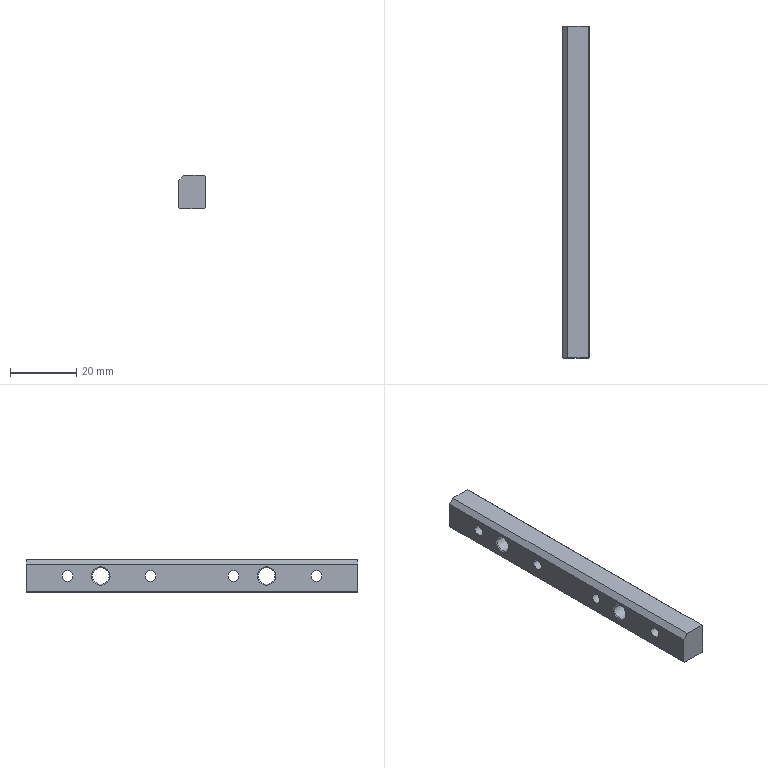Part | NX | 1 solid | 38 faces | box 8 x 100 x 10 mm | volume 7277 mm3 | cone 16 | cylinder 12 | plane 10 | commonest cylinder face diameters 3.3 x8 5 x4
STEP:
#1=CARTESIAN_POINT('',(7.7,0.,0.));
#2=VERTEX_POINT('',#1);
#3=CARTESIAN_POINT('',(1.5,0.,0.));
#4=VERTEX_POINT('',#3);
#5=CARTESIAN_POINT('',(8.,0.,0.));
#6=DIRECTION('',(-1.,0.,0.));
#7=VECTOR('',#6,1000.);
#8=LINE('',#5,#7);
#9=EDGE_CURVE('',#2,#4,#8,.T.);
#10=ORIENTED_EDGE('',*,*,#9,.T.);
#11=CARTESIAN_POINT('',(0.,0.,-1.5));
#12=VERTEX_POINT('',#11);
#13=CARTESIAN_POINT('',(0.,0.,-1.5));
#14=DIRECTION('',(0.7071,0.,0.7071));
#15=VECTOR('',#14,1000.);
#16=LINE('',#13,#15);
#17=EDGE_CURVE('',#12,#4,#16,.T.);
#18=ORIENTED_EDGE('',*,*,#17,.F.);
#19=CARTESIAN_POINT('',(0.,0.,-9.7));
#20=VERTEX_POINT('',#19);
#21=CARTESIAN_POINT('',(0.,0.,0.));
#22=DIRECTION('',(0.,0.,1.));
#23=VECTOR('',#22,1000.);
#24=LINE('',#21,#23);
#25=EDGE_CURVE('',#20,#12,#24,.T.);
#26=ORIENTED_EDGE('',*,*,#25,.F.);
#27=CARTESIAN_POINT('',(0.3,0.,-10.));
#28=VERTEX_POINT('',#27);
#29=CARTESIAN_POINT('',(-9.7,0.,0.));
#30=DIRECTION('',(-0.7071,0.,0.7071));
#31=VECTOR('',#30,1000.);
#32=LINE('',#29,#31);
#33=EDGE_CURVE('',#28,#20,#32,.T.);
#34=ORIENTED_EDGE('',*,*,#33,.F.);
#35=CARTESIAN_POINT('',(7.7,0.,-10.));
#36=VERTEX_POINT('',#35);
#37=CARTESIAN_POINT('',(0.,0.,-10.));
#38=DIRECTION('',(1.,0.,0.));
#39=VECTOR('',#38,1000.);
#40=LINE('',#37,#39);
#41=EDGE_CURVE('',#28,#36,#40,.T.);
#42=ORIENTED_EDGE('',*,*,#41,.T.);
#43=CARTESIAN_POINT('',(8.,0.,-9.7));
#44=VERTEX_POINT('',#43);
#45=CARTESIAN_POINT('',(17.7,0.,0.));
#46=DIRECTION('',(0.7071,0.,0.7071));
#47=VECTOR('',#46,1000.);
#48=LINE('',#45,#47);
#49=EDGE_CURVE('',#36,#44,#48,.T.);
#50=ORIENTED_EDGE('',*,*,#49,.T.);
#51=CARTESIAN_POINT('',(8.,0.,-0.3));
#52=VERTEX_POINT('',#51);
#53=CARTESIAN_POINT('',(8.,0.,0.));
#54=DIRECTION('',(0.,0.,-1.));
#55=VECTOR('',#54,1000.);
#56=LINE('',#53,#55);
#57=EDGE_CURVE('',#52,#44,#56,.T.);
#58=ORIENTED_EDGE('',*,*,#57,.F.);
#59=CARTESIAN_POINT('',(7.7,0.,0.));
#60=DIRECTION('',(-0.7071,0.,0.7071));
#61=VECTOR('',#60,1000.);
#62=LINE('',#59,#61);
#63=EDGE_CURVE('',#52,#2,#62,.T.);
#64=ORIENTED_EDGE('',*,*,#63,.T.);
#65=EDGE_LOOP('',(#10,#18,#26,#34,#42,#50,#58,#64));
#66=FACE_BOUND('',#65,.T.);
#67=CARTESIAN_POINT('',(0.,0.,0.));
#68=DIRECTION('',(0.,1.,0.));
#69=DIRECTION('',(1.,0.,0.));
#70=AXIS2_PLACEMENT_3D('',#67,#68,#69);
#71=PLANE('',#70);
#72=ADVANCED_FACE('',(#66),#71,.F.);
#73=CARTESIAN_POINT('',(7.7,100.,0.));
#74=VERTEX_POINT('',#73);
#75=CARTESIAN_POINT('',(7.7,0.,0.));
#76=DIRECTION('',(0.,-1.,0.));
#77=VECTOR('',#76,1000.);
#78=LINE('',#75,#77);
#79=EDGE_CURVE('',#74,#2,#78,.T.);
#80=ORIENTED_EDGE('',*,*,#79,.F.);
#81=CARTESIAN_POINT('',(1.5,100.,0.));
#82=VERTEX_POINT('',#81);
#83=CARTESIAN_POINT('',(8.,100.,0.));
#84=DIRECTION('',(-1.,0.,0.));
#85=VECTOR('',#84,1000.);
#86=LINE('',#83,#85);
#87=EDGE_CURVE('',#74,#82,#86,.T.);
#88=ORIENTED_EDGE('',*,*,#87,.T.);
#89=CARTESIAN_POINT('',(1.5,100.,0.));
#90=DIRECTION('',(0.,-1.,0.));
#91=VECTOR('',#90,1000.);
#92=LINE('',#89,#91);
#93=EDGE_CURVE('',#82,#4,#92,.T.);
#94=ORIENTED_EDGE('',*,*,#93,.T.);
#95=ORIENTED_EDGE('',*,*,#9,.F.);
#96=EDGE_LOOP('',(#80,#88,#94,#95));
#97=FACE_BOUND('',#96,.T.);
#98=CARTESIAN_POINT('',(0.,0.,0.));
#99=DIRECTION('',(0.,0.,1.));
#100=DIRECTION('',(1.,0.,0.));
#101=AXIS2_PLACEMENT_3D('',#98,#99,#100);
#102=PLANE('',#101);
#103=ADVANCED_FACE('',(#97),#102,.T.);
#104=ORIENTED_EDGE('',*,*,#93,.F.);
#105=CARTESIAN_POINT('',(0.,100.,-1.5));
#106=VERTEX_POINT('',#105);
#107=CARTESIAN_POINT('',(1.5,100.,0.));
#108=DIRECTION('',(-0.7071,0.,-0.7071));
#109=VECTOR('',#108,1000.);
#110=LINE('',#107,#109);
#111=EDGE_CURVE('',#82,#106,#110,.T.);
#112=ORIENTED_EDGE('',*,*,#111,.T.);
#113=CARTESIAN_POINT('',(0.,0.,-1.5));
#114=DIRECTION('',(0.,-1.,0.));
#115=VECTOR('',#114,1000.);
#116=LINE('',#113,#115);
#117=EDGE_CURVE('',#106,#12,#116,.T.);
#118=ORIENTED_EDGE('',*,*,#117,.T.);
#119=ORIENTED_EDGE('',*,*,#17,.T.);
#120=EDGE_LOOP('',(#104,#112,#118,#119));
#121=FACE_BOUND('',#120,.T.);
#122=CARTESIAN_POINT('',(1.5,0.,0.));
#123=DIRECTION('',(-0.7071,0.,0.7071));
#124=DIRECTION('',(0.,1.,0.));
#125=AXIS2_PLACEMENT_3D('',#122,#123,#124);
#126=PLANE('',#125);
#127=ADVANCED_FACE('',(#121),#126,.T.);
#128=ORIENTED_EDGE('',*,*,#57,.T.);
#129=CARTESIAN_POINT('',(8.,100.,-9.7));
#130=VERTEX_POINT('',#129);
#131=CARTESIAN_POINT('',(8.,0.,-9.7));
#132=DIRECTION('',(0.,-1.,0.));
#133=VECTOR('',#132,1000.);
#134=LINE('',#131,#133);
#135=EDGE_CURVE('',#130,#44,#134,.T.);
#136=ORIENTED_EDGE('',*,*,#135,.F.);
#137=CARTESIAN_POINT('',(8.,100.,-0.3));
#138=VERTEX_POINT('',#137);
#139=CARTESIAN_POINT('',(8.,100.,0.));
#140=DIRECTION('',(0.,0.,-1.));
#141=VECTOR('',#140,1000.);
#142=LINE('',#139,#141);
#143=EDGE_CURVE('',#138,#130,#142,.T.);
#144=ORIENTED_EDGE('',*,*,#143,.F.);
#145=CARTESIAN_POINT('',(8.,0.,-0.3));
#146=DIRECTION('',(0.,1.,0.));
#147=VECTOR('',#146,1000.);
#148=LINE('',#145,#147);
#149=EDGE_CURVE('',#52,#138,#148,.T.);
#150=ORIENTED_EDGE('',*,*,#149,.F.);
#151=EDGE_LOOP('',(#128,#136,#144,#150));
#152=FACE_BOUND('',#151,.T.);
#153=CARTESIAN_POINT('',(8.,30.3,-5.));
#154=VERTEX_POINT('',#153);
#155=CARTESIAN_POINT('',(8.,24.7,-5.));
#156=VERTEX_POINT('',#155);
#157=CARTESIAN_POINT('',(8.,27.5,-5.));
#158=DIRECTION('',(1.,0.,0.));
#159=DIRECTION('',(0.,-1.,0.));
#160=AXIS2_PLACEMENT_3D('',#157,#158,#159);
#161=CIRCLE('',#160,2.8);
#162=EDGE_CURVE('',#154,#156,#161,.T.);
#163=ORIENTED_EDGE('',*,*,#162,.F.);
#164=CARTESIAN_POINT('',(8.,27.5,-5.));
#165=DIRECTION('',(1.,0.,0.));
#166=DIRECTION('',(0.,-1.,0.));
#167=AXIS2_PLACEMENT_3D('',#164,#165,#166);
#168=CIRCLE('',#167,2.8);
#169=EDGE_CURVE('',#156,#154,#168,.T.);
#170=ORIENTED_EDGE('',*,*,#169,.F.);
#171=EDGE_LOOP('',(#163,#170));
#172=FACE_BOUND('',#171,.T.);
#173=CARTESIAN_POINT('',(8.,89.815,-5.));
#174=VERTEX_POINT('',#173);
#175=CARTESIAN_POINT('',(8.,85.185,-5.));
#176=VERTEX_POINT('',#175);
#177=CARTESIAN_POINT('',(8.,87.5,-5.));
#178=DIRECTION('',(1.,0.,0.));
#179=DIRECTION('',(0.,-1.,0.));
#180=AXIS2_PLACEMENT_3D('',#177,#178,#179);
#181=CIRCLE('',#180,2.315);
#182=EDGE_CURVE('',#174,#176,#181,.T.);
#183=ORIENTED_EDGE('',*,*,#182,.F.);
#184=CARTESIAN_POINT('',(8.,87.5,-5.));
#185=DIRECTION('',(1.,0.,0.));
#186=DIRECTION('',(0.,-1.,0.));
#187=AXIS2_PLACEMENT_3D('',#184,#185,#186);
#188=CIRCLE('',#187,2.315);
#189=EDGE_CURVE('',#176,#174,#188,.T.);
#190=ORIENTED_EDGE('',*,*,#189,.F.);
#191=EDGE_LOOP('',(#183,#190));
#192=FACE_BOUND('',#191,.T.);
#193=CARTESIAN_POINT('',(8.,64.815,-5.));
#194=VERTEX_POINT('',#193);
#195=CARTESIAN_POINT('',(8.,60.185,-5.));
#196=VERTEX_POINT('',#195);
#197=CARTESIAN_POINT('',(8.,62.5,-5.));
#198=DIRECTION('',(1.,0.,0.));
#199=DIRECTION('',(0.,-1.,0.));
#200=AXIS2_PLACEMENT_3D('',#197,#198,#199);
#201=CIRCLE('',#200,2.315);
#202=EDGE_CURVE('',#194,#196,#201,.T.);
#203=ORIENTED_EDGE('',*,*,#202,.F.);
#204=CARTESIAN_POINT('',(8.,62.5,-5.));
#205=DIRECTION('',(1.,0.,0.));
#206=DIRECTION('',(0.,-1.,0.));
#207=AXIS2_PLACEMENT_3D('',#204,#205,#206);
#208=CIRCLE('',#207,2.315);
#209=EDGE_CURVE('',#196,#194,#208,.T.);
#210=ORIENTED_EDGE('',*,*,#209,.F.);
#211=EDGE_LOOP('',(#203,#210));
#212=FACE_BOUND('',#211,.T.);
#213=CARTESIAN_POINT('',(8.,35.185,-5.));
#214=VERTEX_POINT('',#213);
#215=CARTESIAN_POINT('',(8.,39.815,-5.));
#216=VERTEX_POINT('',#215);
#217=CARTESIAN_POINT('',(8.,37.5,-5.));
#218=DIRECTION('',(1.,0.,0.));
#219=DIRECTION('',(0.,-1.,0.));
#220=AXIS2_PLACEMENT_3D('',#217,#218,#219);
#221=CIRCLE('',#220,2.315);
#222=EDGE_CURVE('',#214,#216,#221,.T.);
#223=ORIENTED_EDGE('',*,*,#222,.F.);
#224=CARTESIAN_POINT('',(8.,37.5,-5.));
#225=DIRECTION('',(1.,0.,0.));
#226=DIRECTION('',(0.,-1.,0.));
#227=AXIS2_PLACEMENT_3D('',#224,#225,#226);
#228=CIRCLE('',#227,2.315);
#229=EDGE_CURVE('',#216,#214,#228,.T.);
#230=ORIENTED_EDGE('',*,*,#229,.F.);
#231=EDGE_LOOP('',(#223,#230));
#232=FACE_BOUND('',#231,.T.);
#233=CARTESIAN_POINT('',(8.,14.815,-5.));
#234=VERTEX_POINT('',#233);
#235=CARTESIAN_POINT('',(8.,10.185,-5.));
#236=VERTEX_POINT('',#235);
#237=CARTESIAN_POINT('',(8.,12.5,-5.));
#238=DIRECTION('',(1.,0.,0.));
#239=DIRECTION('',(0.,-1.,0.));
#240=AXIS2_PLACEMENT_3D('',#237,#238,#239);
#241=CIRCLE('',#240,2.315);
#242=EDGE_CURVE('',#234,#236,#241,.T.);
#243=ORIENTED_EDGE('',*,*,#242,.F.);
#244=CARTESIAN_POINT('',(8.,12.5,-5.));
#245=DIRECTION('',(1.,0.,0.));
#246=DIRECTION('',(0.,-1.,0.));
#247=AXIS2_PLACEMENT_3D('',#244,#245,#246);
#248=CIRCLE('',#247,2.315);
#249=EDGE_CURVE('',#236,#234,#248,.T.);
#250=ORIENTED_EDGE('',*,*,#249,.F.);
#251=EDGE_LOOP('',(#243,#250));
#252=FACE_BOUND('',#251,.T.);
#253=CARTESIAN_POINT('',(8.,80.3,-5.));
#254=VERTEX_POINT('',#253);
#255=CARTESIAN_POINT('',(8.,74.7,-5.));
#256=VERTEX_POINT('',#255);
#257=CARTESIAN_POINT('',(8.,77.5,-5.));
#258=DIRECTION('',(1.,0.,0.));
#259=DIRECTION('',(0.,-1.,0.));
#260=AXIS2_PLACEMENT_3D('',#257,#258,#259);
#261=CIRCLE('',#260,2.8);
#262=EDGE_CURVE('',#254,#256,#261,.T.);
#263=ORIENTED_EDGE('',*,*,#262,.F.);
#264=CARTESIAN_POINT('',(8.,77.5,-5.));
#265=DIRECTION('',(1.,0.,0.));
#266=DIRECTION('',(0.,-1.,0.));
#267=AXIS2_PLACEMENT_3D('',#264,#265,#266);
#268=CIRCLE('',#267,2.8);
#269=EDGE_CURVE('',#256,#254,#268,.T.);
#270=ORIENTED_EDGE('',*,*,#269,.F.);
#271=EDGE_LOOP('',(#263,#270));
#272=FACE_BOUND('',#271,.T.);
#273=CARTESIAN_POINT('',(8.,0.,0.));
#274=DIRECTION('',(1.,0.,0.));
#275=DIRECTION('',(0.,1.,0.));
#276=AXIS2_PLACEMENT_3D('',#273,#274,#275);
#277=PLANE('',#276);
#278=ADVANCED_FACE('',(#152,#172,#192,#212,#232,#252,#272),#277,.T.);
#279=CARTESIAN_POINT('',(7.7,100.,-10.));
#280=VERTEX_POINT('',#279);
#281=CARTESIAN_POINT('',(7.7,0.,-10.));
#282=DIRECTION('',(0.,1.,0.));
#283=VECTOR('',#282,1000.);
#284=LINE('',#281,#283);
#285=EDGE_CURVE('',#36,#280,#284,.T.);
#286=ORIENTED_EDGE('',*,*,#285,.F.);
#287=ORIENTED_EDGE('',*,*,#41,.F.);
#288=CARTESIAN_POINT('',(0.3,100.,-10.));
#289=VERTEX_POINT('',#288);
#290=CARTESIAN_POINT('',(0.3,0.,-10.));
#291=DIRECTION('',(0.,1.,0.));
#292=VECTOR('',#291,1000.);
#293=LINE('',#290,#292);
#294=EDGE_CURVE('',#28,#289,#293,.T.);
#295=ORIENTED_EDGE('',*,*,#294,.T.);
#296=CARTESIAN_POINT('',(0.,100.,-10.));
#297=DIRECTION('',(1.,0.,0.));
#298=VECTOR('',#297,1000.);
#299=LINE('',#296,#298);
#300=EDGE_CURVE('',#289,#280,#299,.T.);
#301=ORIENTED_EDGE('',*,*,#300,.T.);
#302=EDGE_LOOP('',(#286,#287,#295,#301));
#303=FACE_BOUND('',#302,.T.);
#304=CARTESIAN_POINT('',(8.,0.,-10.));
#305=DIRECTION('',(0.,0.,-1.));
#306=DIRECTION('',(0.,-1.,0.));
#307=AXIS2_PLACEMENT_3D('',#304,#305,#306);
#308=PLANE('',#307);
#309=ADVANCED_FACE('',(#303),#308,.T.);
#310=CARTESIAN_POINT('',(0.,100.,-9.7));
#311=VERTEX_POINT('',#310);
#312=CARTESIAN_POINT('',(0.,0.,-9.7));
#313=DIRECTION('',(0.,-1.,0.));
#314=VECTOR('',#313,1000.);
#315=LINE('',#312,#314);
#316=EDGE_CURVE('',#311,#20,#315,.T.);
#317=ORIENTED_EDGE('',*,*,#316,.T.);
#318=ORIENTED_EDGE('',*,*,#25,.T.);
#319=ORIENTED_EDGE('',*,*,#117,.F.);
#320=CARTESIAN_POINT('',(0.,100.,0.));
#321=DIRECTION('',(0.,0.,1.));
#322=VECTOR('',#321,1000.);
#323=LINE('',#320,#322);
#324=EDGE_CURVE('',#311,#106,#323,.T.);
#325=ORIENTED_EDGE('',*,*,#324,.F.);
#326=EDGE_LOOP('',(#317,#318,#319,#325));
#327=FACE_BOUND('',#326,.T.);
#328=CARTESIAN_POINT('',(0.,24.7,-5.));
#329=VERTEX_POINT('',#328);
#330=CARTESIAN_POINT('',(0.,30.3,-5.));
#331=VERTEX_POINT('',#330);
#332=CARTESIAN_POINT('',(0.,27.5,-5.));
#333=DIRECTION('',(-1.,0.,0.));
#334=DIRECTION('',(0.,1.,0.));
#335=AXIS2_PLACEMENT_3D('',#332,#333,#334);
#336=CIRCLE('',#335,2.8);
#337=EDGE_CURVE('',#329,#331,#336,.T.);
#338=ORIENTED_EDGE('',*,*,#337,.F.);
#339=CARTESIAN_POINT('',(0.,27.5,-5.));
#340=DIRECTION('',(-1.,0.,0.));
#341=DIRECTION('',(0.,1.,0.));
#342=AXIS2_PLACEMENT_3D('',#339,#340,#341);
#343=CIRCLE('',#342,2.8);
#344=EDGE_CURVE('',#331,#329,#343,.T.);
#345=ORIENTED_EDGE('',*,*,#344,.F.);
#346=EDGE_LOOP('',(#338,#345));
#347=FACE_BOUND('',#346,.T.);
#348=CARTESIAN_POINT('',(0.,14.15,-5.));
#349=VERTEX_POINT('',#348);
#350=CARTESIAN_POINT('',(0.,10.85,-5.));
#351=VERTEX_POINT('',#350);
#352=CARTESIAN_POINT('',(0.,12.5,-5.));
#353=DIRECTION('',(1.,0.,0.));
#354=DIRECTION('',(0.,-1.,0.));
#355=AXIS2_PLACEMENT_3D('',#352,#353,#354);
#356=CIRCLE('',#355,1.65);
#357=EDGE_CURVE('',#349,#351,#356,.T.);
#358=ORIENTED_EDGE('',*,*,#357,.T.);
#359=CARTESIAN_POINT('',(0.,12.5,-5.));
#360=DIRECTION('',(1.,0.,0.));
#361=DIRECTION('',(0.,-1.,0.));
#362=AXIS2_PLACEMENT_3D('',#359,#360,#361);
#363=CIRCLE('',#362,1.65);
#364=EDGE_CURVE('',#351,#349,#363,.T.);
#365=ORIENTED_EDGE('',*,*,#364,.T.);
#366=EDGE_LOOP('',(#358,#365));
#367=FACE_BOUND('',#366,.T.);
#368=CARTESIAN_POINT('',(0.,39.15,-5.));
#369=VERTEX_POINT('',#368);
#370=CARTESIAN_POINT('',(0.,35.85,-5.));
#371=VERTEX_POINT('',#370);
#372=CARTESIAN_POINT('',(0.,37.5,-5.));
#373=DIRECTION('',(1.,0.,0.));
#374=DIRECTION('',(0.,-1.,0.));
#375=AXIS2_PLACEMENT_3D('',#372,#373,#374);
#376=CIRCLE('',#375,1.65);
#377=EDGE_CURVE('',#369,#371,#376,.T.);
#378=ORIENTED_EDGE('',*,*,#377,.T.);
#379=CARTESIAN_POINT('',(0.,37.5,-5.));
#380=DIRECTION('',(1.,0.,0.));
#381=DIRECTION('',(0.,-1.,0.));
#382=AXIS2_PLACEMENT_3D('',#379,#380,#381);
#383=CIRCLE('',#382,1.65);
#384=EDGE_CURVE('',#371,#369,#383,.T.);
#385=ORIENTED_EDGE('',*,*,#384,.T.);
#386=EDGE_LOOP('',(#378,#385));
#387=FACE_BOUND('',#386,.T.);
#388=CARTESIAN_POINT('',(0.,60.85,-5.));
#389=VERTEX_POINT('',#388);
#390=CARTESIAN_POINT('',(0.,64.15,-5.));
#391=VERTEX_POINT('',#390);
#392=CARTESIAN_POINT('',(0.,62.5,-5.));
#393=DIRECTION('',(1.,0.,0.));
#394=DIRECTION('',(0.,-1.,0.));
#395=AXIS2_PLACEMENT_3D('',#392,#393,#394);
#396=CIRCLE('',#395,1.65);
#397=EDGE_CURVE('',#389,#391,#396,.T.);
#398=ORIENTED_EDGE('',*,*,#397,.T.);
#399=CARTESIAN_POINT('',(0.,62.5,-5.));
#400=DIRECTION('',(1.,0.,0.));
#401=DIRECTION('',(0.,-1.,0.));
#402=AXIS2_PLACEMENT_3D('',#399,#400,#401);
#403=CIRCLE('',#402,1.65);
#404=EDGE_CURVE('',#391,#389,#403,.T.);
#405=ORIENTED_EDGE('',*,*,#404,.T.);
#406=EDGE_LOOP('',(#398,#405));
#407=FACE_BOUND('',#406,.T.);
#408=CARTESIAN_POINT('',(0.,80.3,-5.));
#409=VERTEX_POINT('',#408);
#410=CARTESIAN_POINT('',(0.,74.7,-5.));
#411=VERTEX_POINT('',#410);
#412=CARTESIAN_POINT('',(0.,77.5,-5.));
#413=DIRECTION('',(-1.,0.,0.));
#414=DIRECTION('',(0.,1.,0.));
#415=AXIS2_PLACEMENT_3D('',#412,#413,#414);
#416=CIRCLE('',#415,2.8);
#417=EDGE_CURVE('',#409,#411,#416,.T.);
#418=ORIENTED_EDGE('',*,*,#417,.F.);
#419=CARTESIAN_POINT('',(0.,77.5,-5.));
#420=DIRECTION('',(-1.,0.,0.));
#421=DIRECTION('',(0.,1.,0.));
#422=AXIS2_PLACEMENT_3D('',#419,#420,#421);
#423=CIRCLE('',#422,2.8);
#424=EDGE_CURVE('',#411,#409,#423,.T.);
#425=ORIENTED_EDGE('',*,*,#424,.F.);
#426=EDGE_LOOP('',(#418,#425));
#427=FACE_BOUND('',#426,.T.);
#428=CARTESIAN_POINT('',(0.,89.15,-5.));
#429=VERTEX_POINT('',#428);
#430=CARTESIAN_POINT('',(0.,85.85,-5.));
#431=VERTEX_POINT('',#430);
#432=CARTESIAN_POINT('',(0.,87.5,-5.));
#433=DIRECTION('',(1.,0.,0.));
#434=DIRECTION('',(0.,-1.,0.));
#435=AXIS2_PLACEMENT_3D('',#432,#433,#434);
#436=CIRCLE('',#435,1.65);
#437=EDGE_CURVE('',#429,#431,#436,.T.);
#438=ORIENTED_EDGE('',*,*,#437,.T.);
#439=CARTESIAN_POINT('',(0.,87.5,-5.));
#440=DIRECTION('',(1.,0.,0.));
#441=DIRECTION('',(0.,-1.,0.));
#442=AXIS2_PLACEMENT_3D('',#439,#440,#441);
#443=CIRCLE('',#442,1.65);
#444=EDGE_CURVE('',#431,#429,#443,.T.);
#445=ORIENTED_EDGE('',*,*,#444,.T.);
#446=EDGE_LOOP('',(#438,#445));
#447=FACE_BOUND('',#446,.T.);
#448=CARTESIAN_POINT('',(0.,0.,-10.));
#449=DIRECTION('',(-1.,0.,0.));
#450=DIRECTION('',(0.,0.,1.));
#451=AXIS2_PLACEMENT_3D('',#448,#449,#450);
#452=PLANE('',#451);
#453=ADVANCED_FACE('',(#327,#347,#367,#387,#407,#427,#447),#452,.T.);
#454=ORIENTED_EDGE('',*,*,#87,.F.);
#455=CARTESIAN_POINT('',(7.7,100.,0.));
#456=DIRECTION('',(-0.7071,0.,0.7071));
#457=VECTOR('',#456,1000.);
#458=LINE('',#455,#457);
#459=EDGE_CURVE('',#138,#74,#458,.T.);
#460=ORIENTED_EDGE('',*,*,#459,.F.);
#461=ORIENTED_EDGE('',*,*,#143,.T.);
#462=CARTESIAN_POINT('',(17.7,100.,0.));
#463=DIRECTION('',(0.7071,0.,0.7071));
#464=VECTOR('',#463,1000.);
#465=LINE('',#462,#464);
#466=EDGE_CURVE('',#280,#130,#465,.T.);
#467=ORIENTED_EDGE('',*,*,#466,.F.);
#468=ORIENTED_EDGE('',*,*,#300,.F.);
#469=CARTESIAN_POINT('',(-9.7,100.,0.));
#470=DIRECTION('',(-0.7071,0.,0.7071));
#471=VECTOR('',#470,1000.);
#472=LINE('',#469,#471);
#473=EDGE_CURVE('',#289,#311,#472,.T.);
#474=ORIENTED_EDGE('',*,*,#473,.T.);
#475=ORIENTED_EDGE('',*,*,#324,.T.);
#476=ORIENTED_EDGE('',*,*,#111,.F.);
#477=EDGE_LOOP('',(#454,#460,#461,#467,#468,#474,#475,#476));
#478=FACE_BOUND('',#477,.T.);
#479=CARTESIAN_POINT('',(0.,100.,0.));
#480=DIRECTION('',(0.,1.,0.));
#481=DIRECTION('',(1.,0.,0.));
#482=AXIS2_PLACEMENT_3D('',#479,#480,#481);
#483=PLANE('',#482);
#484=ADVANCED_FACE('',(#478),#483,.T.);
#485=CARTESIAN_POINT('',(7.7,25.,-5.));
#486=VERTEX_POINT('',#485);
#487=CARTESIAN_POINT('',(7.7,30.,-5.));
#488=VERTEX_POINT('',#487);
#489=CARTESIAN_POINT('',(7.7,27.5,-5.));
#490=DIRECTION('',(1.,0.,0.));
#491=DIRECTION('',(0.,-1.,0.));
#492=AXIS2_PLACEMENT_3D('',#489,#490,#491);
#493=CIRCLE('',#492,2.5);
#494=EDGE_CURVE('',#486,#488,#493,.T.);
#495=ORIENTED_EDGE('',*,*,#494,.T.);
#496=CARTESIAN_POINT('',(0.3,30.,-5.));
#497=VERTEX_POINT('',#496);
#498=CARTESIAN_POINT('',(0.,30.,-5.));
#499=DIRECTION('',(1.,0.,0.));
#500=VECTOR('',#499,1000.);
#501=LINE('',#498,#500);
#502=EDGE_CURVE('',#497,#488,#501,.T.);
#503=ORIENTED_EDGE('',*,*,#502,.F.);
#504=CARTESIAN_POINT('',(0.3,25.,-5.));
#505=VERTEX_POINT('',#504);
#506=CARTESIAN_POINT('',(0.3,27.5,-5.));
#507=DIRECTION('',(-1.,0.,0.));
#508=DIRECTION('',(0.,1.,0.));
#509=AXIS2_PLACEMENT_3D('',#506,#507,#508);
#510=CIRCLE('',#509,2.5);
#511=EDGE_CURVE('',#497,#505,#510,.T.);
#512=ORIENTED_EDGE('',*,*,#511,.T.);
#513=CARTESIAN_POINT('',(0.,25.,-5.));
#514=DIRECTION('',(1.,0.,0.));
#515=VECTOR('',#514,1000.);
#516=LINE('',#513,#515);
#517=EDGE_CURVE('',#505,#486,#516,.T.);
#518=ORIENTED_EDGE('',*,*,#517,.T.);
#519=EDGE_LOOP('',(#495,#503,#512,#518));
#520=FACE_BOUND('',#519,.T.);
#521=CARTESIAN_POINT('',(0.,27.5,-5.));
#522=DIRECTION('',(1.,0.,0.));
#523=DIRECTION('',(0.,1.,0.));
#524=AXIS2_PLACEMENT_3D('',#521,#522,#523);
#525=CYLINDRICAL_SURFACE('',#524,2.5);
#526=ADVANCED_FACE('',(#520),#525,.F.);
#527=CARTESIAN_POINT('',(7.7,75.,-5.));
#528=VERTEX_POINT('',#527);
#529=CARTESIAN_POINT('',(7.7,80.,-5.));
#530=VERTEX_POINT('',#529);
#531=CARTESIAN_POINT('',(7.7,77.5,-5.));
#532=DIRECTION('',(1.,0.,0.));
#533=DIRECTION('',(0.,-1.,0.));
#534=AXIS2_PLACEMENT_3D('',#531,#532,#533);
#535=CIRCLE('',#534,2.5);
#536=EDGE_CURVE('',#528,#530,#535,.T.);
#537=ORIENTED_EDGE('',*,*,#536,.T.);
#538=CARTESIAN_POINT('',(0.3,80.,-5.));
#539=VERTEX_POINT('',#538);
#540=CARTESIAN_POINT('',(0.,80.,-5.));
#541=DIRECTION('',(1.,0.,0.));
#542=VECTOR('',#541,1000.);
#543=LINE('',#540,#542);
#544=EDGE_CURVE('',#539,#530,#543,.T.);
#545=ORIENTED_EDGE('',*,*,#544,.F.);
#546=CARTESIAN_POINT('',(0.3,75.,-5.));
#547=VERTEX_POINT('',#546);
#548=CARTESIAN_POINT('',(0.3,77.5,-5.));
#549=DIRECTION('',(-1.,0.,0.));
#550=DIRECTION('',(0.,1.,0.));
#551=AXIS2_PLACEMENT_3D('',#548,#549,#550);
#552=CIRCLE('',#551,2.5);
#553=EDGE_CURVE('',#539,#547,#552,.T.);
#554=ORIENTED_EDGE('',*,*,#553,.T.);
#555=CARTESIAN_POINT('',(0.,75.,-5.));
#556=DIRECTION('',(1.,0.,0.));
#557=VECTOR('',#556,1000.);
#558=LINE('',#555,#557);
#559=EDGE_CURVE('',#547,#528,#558,.T.);
#560=ORIENTED_EDGE('',*,*,#559,.T.);
#561=EDGE_LOOP('',(#537,#545,#554,#560));
#562=FACE_BOUND('',#561,.T.);
#563=CARTESIAN_POINT('',(0.,77.5,-5.));
#564=DIRECTION('',(1.,0.,0.));
#565=DIRECTION('',(0.,1.,0.));
#566=AXIS2_PLACEMENT_3D('',#563,#564,#565);
#567=CYLINDRICAL_SURFACE('',#566,2.5);
#568=ADVANCED_FACE('',(#562),#567,.F.);
#569=ORIENTED_EDGE('',*,*,#262,.T.);
#570=CARTESIAN_POINT('',(8.,74.7,-5.));
#571=DIRECTION('',(0.7071,-0.7071,0.));
#572=VECTOR('',#571,1000.);
#573=LINE('',#570,#572);
#574=EDGE_CURVE('',#256,#528,#573,.F.);
#575=ORIENTED_EDGE('',*,*,#574,.T.);
#576=CARTESIAN_POINT('',(7.7,77.5,-5.));
#577=DIRECTION('',(1.,0.,0.));
#578=DIRECTION('',(0.,-1.,0.));
#579=AXIS2_PLACEMENT_3D('',#576,#577,#578);
#580=CIRCLE('',#579,2.5);
#581=EDGE_CURVE('',#530,#528,#580,.T.);
#582=ORIENTED_EDGE('',*,*,#581,.F.);
#583=CARTESIAN_POINT('',(8.,80.3,-5.));
#584=DIRECTION('',(0.7071,0.7071,0.));
#585=VECTOR('',#584,1000.);
#586=LINE('',#583,#585);
#587=EDGE_CURVE('',#254,#530,#586,.F.);
#588=ORIENTED_EDGE('',*,*,#587,.F.);
#589=EDGE_LOOP('',(#569,#575,#582,#588));
#590=FACE_BOUND('',#589,.T.);
#591=CARTESIAN_POINT('',(8.,77.5,-5.));
#592=DIRECTION('',(1.,0.,0.));
#593=DIRECTION('',(0.,-1.,0.));
#594=AXIS2_PLACEMENT_3D('',#591,#592,#593);
#595=CONICAL_SURFACE('',#594,2.8,0.7854);
#596=ADVANCED_FACE('',(#590),#595,.F.);
#597=ORIENTED_EDGE('',*,*,#377,.F.);
#598=CARTESIAN_POINT('',(7.616,39.15,-5.));
#599=VERTEX_POINT('',#598);
#600=CARTESIAN_POINT('',(8.,39.15,-5.));
#601=DIRECTION('',(1.,0.,0.));
#602=VECTOR('',#601,1000.);
#603=LINE('',#600,#602);
#604=EDGE_CURVE('',#369,#599,#603,.T.);
#605=ORIENTED_EDGE('',*,*,#604,.T.);
#606=CARTESIAN_POINT('',(7.616,35.85,-5.));
#607=VERTEX_POINT('',#606);
#608=CARTESIAN_POINT('',(7.616,37.5,-5.));
#609=DIRECTION('',(1.,0.,0.));
#610=DIRECTION('',(0.,-1.,0.));
#611=AXIS2_PLACEMENT_3D('',#608,#609,#610);
#612=CIRCLE('',#611,1.65);
#613=EDGE_CURVE('',#599,#607,#612,.T.);
#614=ORIENTED_EDGE('',*,*,#613,.T.);
#615=CARTESIAN_POINT('',(8.,35.85,-5.));
#616=DIRECTION('',(1.,0.,0.));
#617=VECTOR('',#616,1000.);
#618=LINE('',#615,#617);
#619=EDGE_CURVE('',#371,#607,#618,.T.);
#620=ORIENTED_EDGE('',*,*,#619,.F.);
#621=EDGE_LOOP('',(#597,#605,#614,#620));
#622=FACE_BOUND('',#621,.T.);
#623=CARTESIAN_POINT('',(8.,37.5,-5.));
#624=DIRECTION('',(1.,0.,0.));
#625=DIRECTION('',(0.,-1.,0.));
#626=AXIS2_PLACEMENT_3D('',#623,#624,#625);
#627=CYLINDRICAL_SURFACE('',#626,1.65);
#628=ADVANCED_FACE('',(#622),#627,.F.);
#629=ORIENTED_EDGE('',*,*,#222,.T.);
#630=CARTESIAN_POINT('',(7.616,39.15,-5.));
#631=DIRECTION('',(0.5,0.866,0.));
#632=VECTOR('',#631,1000.);
#633=LINE('',#630,#632);
#634=EDGE_CURVE('',#216,#599,#633,.F.);
#635=ORIENTED_EDGE('',*,*,#634,.T.);
#636=CARTESIAN_POINT('',(7.616,37.5,-5.));
#637=DIRECTION('',(1.,0.,0.));
#638=DIRECTION('',(0.,-1.,0.));
#639=AXIS2_PLACEMENT_3D('',#636,#637,#638);
#640=CIRCLE('',#639,1.65);
#641=EDGE_CURVE('',#607,#599,#640,.T.);
#642=ORIENTED_EDGE('',*,*,#641,.F.);
#643=CARTESIAN_POINT('',(7.616,35.85,-5.));
#644=DIRECTION('',(0.5,-0.866,0.));
#645=VECTOR('',#644,1000.);
#646=LINE('',#643,#645);
#647=EDGE_CURVE('',#214,#607,#646,.F.);
#648=ORIENTED_EDGE('',*,*,#647,.F.);
#649=EDGE_LOOP('',(#629,#635,#642,#648));
#650=FACE_BOUND('',#649,.T.);
#651=CARTESIAN_POINT('',(7.616,37.5,-5.));
#652=DIRECTION('',(1.,0.,0.));
#653=DIRECTION('',(0.,-1.,0.));
#654=AXIS2_PLACEMENT_3D('',#651,#652,#653);
#655=CONICAL_SURFACE('',#654,1.65,1.047);
#656=ADVANCED_FACE('',(#650),#655,.F.);
#657=ORIENTED_EDGE('',*,*,#357,.F.);
#658=CARTESIAN_POINT('',(7.616,14.15,-5.));
#659=VERTEX_POINT('',#658);
#660=CARTESIAN_POINT('',(8.,14.15,-5.));
#661=DIRECTION('',(1.,0.,0.));
#662=VECTOR('',#661,1000.);
#663=LINE('',#660,#662);
#664=EDGE_CURVE('',#349,#659,#663,.T.);
#665=ORIENTED_EDGE('',*,*,#664,.T.);
#666=CARTESIAN_POINT('',(7.616,10.85,-5.));
#667=VERTEX_POINT('',#666);
#668=CARTESIAN_POINT('',(7.616,12.5,-5.));
#669=DIRECTION('',(1.,0.,0.));
#670=DIRECTION('',(0.,-1.,0.));
#671=AXIS2_PLACEMENT_3D('',#668,#669,#670);
#672=CIRCLE('',#671,1.65);
#673=EDGE_CURVE('',#659,#667,#672,.T.);
#674=ORIENTED_EDGE('',*,*,#673,.T.);
#675=CARTESIAN_POINT('',(8.,10.85,-5.));
#676=DIRECTION('',(1.,0.,0.));
#677=VECTOR('',#676,1000.);
#678=LINE('',#675,#677);
#679=EDGE_CURVE('',#351,#667,#678,.T.);
#680=ORIENTED_EDGE('',*,*,#679,.F.);
#681=EDGE_LOOP('',(#657,#665,#674,#680));
#682=FACE_BOUND('',#681,.T.);
#683=CARTESIAN_POINT('',(8.,12.5,-5.));
#684=DIRECTION('',(1.,0.,0.));
#685=DIRECTION('',(0.,-1.,0.));
#686=AXIS2_PLACEMENT_3D('',#683,#684,#685);
#687=CYLINDRICAL_SURFACE('',#686,1.65);
#688=ADVANCED_FACE('',(#682),#687,.F.);
#689=CARTESIAN_POINT('',(7.616,12.5,-5.));
#690=DIRECTION('',(1.,0.,0.));
#691=DIRECTION('',(0.,-1.,0.));
#692=AXIS2_PLACEMENT_3D('',#689,#690,#691);
#693=CIRCLE('',#692,1.65);
#694=EDGE_CURVE('',#667,#659,#693,.T.);
#695=ORIENTED_EDGE('',*,*,#694,.F.);
#696=CARTESIAN_POINT('',(7.616,10.85,-5.));
#697=DIRECTION('',(0.5,-0.866,0.));
#698=VECTOR('',#697,1000.);
#699=LINE('',#696,#698);
#700=EDGE_CURVE('',#236,#667,#699,.F.);
#701=ORIENTED_EDGE('',*,*,#700,.F.);
#702=ORIENTED_EDGE('',*,*,#249,.T.);
#703=CARTESIAN_POINT('',(7.616,14.15,-5.));
#704=DIRECTION('',(0.5,0.866,0.));
#705=VECTOR('',#704,1000.);
#706=LINE('',#703,#705);
#707=EDGE_CURVE('',#234,#659,#706,.F.);
#708=ORIENTED_EDGE('',*,*,#707,.T.);
#709=EDGE_LOOP('',(#695,#701,#702,#708));
#710=FACE_BOUND('',#709,.T.);
#711=CARTESIAN_POINT('',(7.616,12.5,-5.));
#712=DIRECTION('',(1.,0.,0.));
#713=DIRECTION('',(0.,-1.,0.));
#714=AXIS2_PLACEMENT_3D('',#711,#712,#713);
#715=CONICAL_SURFACE('',#714,1.65,1.047);
#716=ADVANCED_FACE('',(#710),#715,.F.);
#717=ORIENTED_EDGE('',*,*,#397,.F.);
#718=CARTESIAN_POINT('',(7.616,60.85,-5.));
#719=VERTEX_POINT('',#718);
#720=CARTESIAN_POINT('',(8.,60.85,-5.));
#721=DIRECTION('',(1.,0.,0.));
#722=VECTOR('',#721,1000.);
#723=LINE('',#720,#722);
#724=EDGE_CURVE('',#719,#389,#723,.F.);
#725=ORIENTED_EDGE('',*,*,#724,.F.);
#726=CARTESIAN_POINT('',(7.616,64.15,-5.));
#727=VERTEX_POINT('',#726);
#728=CARTESIAN_POINT('',(7.616,62.5,-5.));
#729=DIRECTION('',(1.,0.,0.));
#730=DIRECTION('',(0.,-1.,0.));
#731=AXIS2_PLACEMENT_3D('',#728,#729,#730);
#732=CIRCLE('',#731,1.65);
#733=EDGE_CURVE('',#719,#727,#732,.T.);
#734=ORIENTED_EDGE('',*,*,#733,.T.);
#735=CARTESIAN_POINT('',(8.,64.15,-5.));
#736=DIRECTION('',(1.,0.,0.));
#737=VECTOR('',#736,1000.);
#738=LINE('',#735,#737);
#739=EDGE_CURVE('',#727,#391,#738,.F.);
#740=ORIENTED_EDGE('',*,*,#739,.T.);
#741=EDGE_LOOP('',(#717,#725,#734,#740));
#742=FACE_BOUND('',#741,.T.);
#743=CARTESIAN_POINT('',(8.,62.5,-5.));
#744=DIRECTION('',(1.,0.,0.));
#745=DIRECTION('',(0.,-1.,0.));
#746=AXIS2_PLACEMENT_3D('',#743,#744,#745);
#747=CYLINDRICAL_SURFACE('',#746,1.65);
#748=ADVANCED_FACE('',(#742),#747,.F.);
#749=ORIENTED_EDGE('',*,*,#733,.F.);
#750=CARTESIAN_POINT('',(7.616,60.85,-5.));
#751=DIRECTION('',(0.5,-0.866,0.));
#752=VECTOR('',#751,1000.);
#753=LINE('',#750,#752);
#754=EDGE_CURVE('',#196,#719,#753,.F.);
#755=ORIENTED_EDGE('',*,*,#754,.F.);
#756=ORIENTED_EDGE('',*,*,#209,.T.);
#757=CARTESIAN_POINT('',(7.616,64.15,-5.));
#758=DIRECTION('',(0.5,0.866,0.));
#759=VECTOR('',#758,1000.);
#760=LINE('',#757,#759);
#761=EDGE_CURVE('',#194,#727,#760,.F.);
#762=ORIENTED_EDGE('',*,*,#761,.T.);
#763=EDGE_LOOP('',(#749,#755,#756,#762));
#764=FACE_BOUND('',#763,.T.);
#765=CARTESIAN_POINT('',(7.616,62.5,-5.));
#766=DIRECTION('',(1.,0.,0.));
#767=DIRECTION('',(0.,-1.,0.));
#768=AXIS2_PLACEMENT_3D('',#765,#766,#767);
#769=CONICAL_SURFACE('',#768,1.65,1.047);
#770=ADVANCED_FACE('',(#764),#769,.F.);
#771=ORIENTED_EDGE('',*,*,#316,.F.);
#772=ORIENTED_EDGE('',*,*,#473,.F.);
#773=ORIENTED_EDGE('',*,*,#294,.F.);
#774=ORIENTED_EDGE('',*,*,#33,.T.);
#775=EDGE_LOOP('',(#771,#772,#773,#774));
#776=FACE_BOUND('',#775,.T.);
#777=CARTESIAN_POINT('',(0.15,50.,-9.85));
#778=DIRECTION('',(0.7071,0.,0.7071));
#779=DIRECTION('',(0.,-1.,0.));
#780=AXIS2_PLACEMENT_3D('',#777,#778,#779);
#781=PLANE('',#780);
#782=ADVANCED_FACE('',(#776),#781,.F.);
#783=ORIENTED_EDGE('',*,*,#285,.T.);
#784=ORIENTED_EDGE('',*,*,#466,.T.);
#785=ORIENTED_EDGE('',*,*,#135,.T.);
#786=ORIENTED_EDGE('',*,*,#49,.F.);
#787=EDGE_LOOP('',(#783,#784,#785,#786));
#788=FACE_BOUND('',#787,.T.);
#789=CARTESIAN_POINT('',(7.85,50.,-9.85));
#790=DIRECTION('',(0.7071,0.,-0.7071));
#791=DIRECTION('',(0.,-1.,0.));
#792=AXIS2_PLACEMENT_3D('',#789,#790,#791);
#793=PLANE('',#792);
#794=ADVANCED_FACE('',(#788),#793,.T.);
#795=ORIENTED_EDGE('',*,*,#79,.T.);
#796=ORIENTED_EDGE('',*,*,#63,.F.);
#797=ORIENTED_EDGE('',*,*,#149,.T.);
#798=ORIENTED_EDGE('',*,*,#459,.T.);
#799=EDGE_LOOP('',(#795,#796,#797,#798));
#800=FACE_BOUND('',#799,.T.);
#801=CARTESIAN_POINT('',(7.85,50.,-0.15));
#802=DIRECTION('',(0.7071,0.,0.7071));
#803=DIRECTION('',(0.,-1.,0.));
#804=AXIS2_PLACEMENT_3D('',#801,#802,#803);
#805=PLANE('',#804);
#806=ADVANCED_FACE('',(#800),#805,.T.);
#807=ORIENTED_EDGE('',*,*,#553,.F.);
#808=CARTESIAN_POINT('',(0.,80.3,-5.));
#809=DIRECTION('',(-0.7071,0.7071,0.));
#810=VECTOR('',#809,1000.);
#811=LINE('',#808,#810);
#812=EDGE_CURVE('',#539,#409,#811,.T.);
#813=ORIENTED_EDGE('',*,*,#812,.T.);
#814=ORIENTED_EDGE('',*,*,#417,.T.);
#815=CARTESIAN_POINT('',(0.,74.7,-5.));
#816=DIRECTION('',(-0.7071,-0.7071,0.));
#817=VECTOR('',#816,1000.);
#818=LINE('',#815,#817);
#819=EDGE_CURVE('',#547,#411,#818,.T.);
#820=ORIENTED_EDGE('',*,*,#819,.F.);
#821=EDGE_LOOP('',(#807,#813,#814,#820));
#822=FACE_BOUND('',#821,.T.);
#823=CARTESIAN_POINT('',(0.,77.5,-5.));
#824=DIRECTION('',(-1.,0.,0.));
#825=DIRECTION('',(0.,1.,0.));
#826=AXIS2_PLACEMENT_3D('',#823,#824,#825);
#827=CONICAL_SURFACE('',#826,2.8,0.7854);
#828=ADVANCED_FACE('',(#822),#827,.F.);
#829=ORIENTED_EDGE('',*,*,#337,.T.);
#830=CARTESIAN_POINT('',(0.,30.3,-5.));
#831=DIRECTION('',(-0.7071,0.7071,0.));
#832=VECTOR('',#831,1000.);
#833=LINE('',#830,#832);
#834=EDGE_CURVE('',#497,#331,#833,.T.);
#835=ORIENTED_EDGE('',*,*,#834,.F.);
#836=CARTESIAN_POINT('',(0.3,27.5,-5.));
#837=DIRECTION('',(-1.,0.,0.));
#838=DIRECTION('',(0.,1.,0.));
#839=AXIS2_PLACEMENT_3D('',#836,#837,#838);
#840=CIRCLE('',#839,2.5);
#841=EDGE_CURVE('',#505,#497,#840,.T.);
#842=ORIENTED_EDGE('',*,*,#841,.F.);
#843=CARTESIAN_POINT('',(0.,24.7,-5.));
#844=DIRECTION('',(-0.7071,-0.7071,0.));
#845=VECTOR('',#844,1000.);
#846=LINE('',#843,#845);
#847=EDGE_CURVE('',#505,#329,#846,.T.);
#848=ORIENTED_EDGE('',*,*,#847,.T.);
#849=EDGE_LOOP('',(#829,#835,#842,#848));
#850=FACE_BOUND('',#849,.T.);
#851=CARTESIAN_POINT('',(0.,27.5,-5.));
#852=DIRECTION('',(-1.,0.,0.));
#853=DIRECTION('',(0.,1.,0.));
#854=AXIS2_PLACEMENT_3D('',#851,#852,#853);
#855=CONICAL_SURFACE('',#854,2.8,0.7854);
#856=ADVANCED_FACE('',(#850),#855,.F.);
#857=ORIENTED_EDGE('',*,*,#494,.F.);
#858=CARTESIAN_POINT('',(8.,24.7,-5.));
#859=DIRECTION('',(0.7071,-0.7071,0.));
#860=VECTOR('',#859,1000.);
#861=LINE('',#858,#860);
#862=EDGE_CURVE('',#156,#486,#861,.F.);
#863=ORIENTED_EDGE('',*,*,#862,.F.);
#864=ORIENTED_EDGE('',*,*,#169,.T.);
#865=CARTESIAN_POINT('',(8.,30.3,-5.));
#866=DIRECTION('',(0.7071,0.7071,0.));
#867=VECTOR('',#866,1000.);
#868=LINE('',#865,#867);
#869=EDGE_CURVE('',#154,#488,#868,.F.);
#870=ORIENTED_EDGE('',*,*,#869,.T.);
#871=EDGE_LOOP('',(#857,#863,#864,#870));
#872=FACE_BOUND('',#871,.T.);
#873=CARTESIAN_POINT('',(8.,27.5,-5.));
#874=DIRECTION('',(1.,0.,0.));
#875=DIRECTION('',(0.,-1.,0.));
#876=AXIS2_PLACEMENT_3D('',#873,#874,#875);
#877=CONICAL_SURFACE('',#876,2.8,0.7854);
#878=ADVANCED_FACE('',(#872),#877,.F.);
#879=CARTESIAN_POINT('',(7.616,85.85,-5.));
#880=VERTEX_POINT('',#879);
#881=CARTESIAN_POINT('',(7.616,89.15,-5.));
#882=VERTEX_POINT('',#881);
#883=CARTESIAN_POINT('',(7.616,87.5,-5.));
#884=DIRECTION('',(1.,0.,0.));
#885=DIRECTION('',(0.,-1.,0.));
#886=AXIS2_PLACEMENT_3D('',#883,#884,#885);
#887=CIRCLE('',#886,1.65);
#888=EDGE_CURVE('',#880,#882,#887,.T.);
#889=ORIENTED_EDGE('',*,*,#888,.T.);
#890=CARTESIAN_POINT('',(8.,89.15,-5.));
#891=DIRECTION('',(1.,0.,0.));
#892=VECTOR('',#891,1000.);
#893=LINE('',#890,#892);
#894=EDGE_CURVE('',#429,#882,#893,.T.);
#895=ORIENTED_EDGE('',*,*,#894,.F.);
#896=ORIENTED_EDGE('',*,*,#444,.F.);
#897=CARTESIAN_POINT('',(8.,85.85,-5.));
#898=DIRECTION('',(1.,0.,0.));
#899=VECTOR('',#898,1000.);
#900=LINE('',#897,#899);
#901=EDGE_CURVE('',#431,#880,#900,.T.);
#902=ORIENTED_EDGE('',*,*,#901,.T.);
#903=EDGE_LOOP('',(#889,#895,#896,#902));
#904=FACE_BOUND('',#903,.T.);
#905=CARTESIAN_POINT('',(8.,87.5,-5.));
#906=DIRECTION('',(1.,0.,0.));
#907=DIRECTION('',(0.,-1.,0.));
#908=AXIS2_PLACEMENT_3D('',#905,#906,#907);
#909=CYLINDRICAL_SURFACE('',#908,1.65);
#910=ADVANCED_FACE('',(#904),#909,.F.);
#911=ORIENTED_EDGE('',*,*,#182,.T.);
#912=CARTESIAN_POINT('',(7.616,85.85,-5.));
#913=DIRECTION('',(0.5,-0.866,0.));
#914=VECTOR('',#913,1000.);
#915=LINE('',#912,#914);
#916=EDGE_CURVE('',#176,#880,#915,.F.);
#917=ORIENTED_EDGE('',*,*,#916,.T.);
#918=CARTESIAN_POINT('',(7.616,87.5,-5.));
#919=DIRECTION('',(1.,0.,0.));
#920=DIRECTION('',(0.,-1.,0.));
#921=AXIS2_PLACEMENT_3D('',#918,#919,#920);
#922=CIRCLE('',#921,1.65);
#923=EDGE_CURVE('',#882,#880,#922,.T.);
#924=ORIENTED_EDGE('',*,*,#923,.F.);
#925=CARTESIAN_POINT('',(7.616,89.15,-5.));
#926=DIRECTION('',(0.5,0.866,0.));
#927=VECTOR('',#926,1000.);
#928=LINE('',#925,#927);
#929=EDGE_CURVE('',#174,#882,#928,.F.);
#930=ORIENTED_EDGE('',*,*,#929,.F.);
#931=EDGE_LOOP('',(#911,#917,#924,#930));
#932=FACE_BOUND('',#931,.T.);
#933=CARTESIAN_POINT('',(7.616,87.5,-5.));
#934=DIRECTION('',(1.,0.,0.));
#935=DIRECTION('',(0.,-1.,0.));
#936=AXIS2_PLACEMENT_3D('',#933,#934,#935);
#937=CONICAL_SURFACE('',#936,1.65,1.047);
#938=ADVANCED_FACE('',(#932),#937,.F.);
#939=ORIENTED_EDGE('',*,*,#888,.F.);
#940=ORIENTED_EDGE('',*,*,#916,.F.);
#941=ORIENTED_EDGE('',*,*,#189,.T.);
#942=ORIENTED_EDGE('',*,*,#929,.T.);
#943=EDGE_LOOP('',(#939,#940,#941,#942));
#944=FACE_BOUND('',#943,.T.);
#945=CARTESIAN_POINT('',(7.616,87.5,-5.));
#946=DIRECTION('',(1.,0.,0.));
#947=DIRECTION('',(0.,-1.,0.));
#948=AXIS2_PLACEMENT_3D('',#945,#946,#947);
#949=CONICAL_SURFACE('',#948,1.65,1.047);
#950=ADVANCED_FACE('',(#944),#949,.F.);
#951=ORIENTED_EDGE('',*,*,#162,.T.);
#952=ORIENTED_EDGE('',*,*,#862,.T.);
#953=CARTESIAN_POINT('',(7.7,27.5,-5.));
#954=DIRECTION('',(1.,0.,0.));
#955=DIRECTION('',(0.,-1.,0.));
#956=AXIS2_PLACEMENT_3D('',#953,#954,#955);
#957=CIRCLE('',#956,2.5);
#958=EDGE_CURVE('',#488,#486,#957,.T.);
#959=ORIENTED_EDGE('',*,*,#958,.F.);
#960=ORIENTED_EDGE('',*,*,#869,.F.);
#961=EDGE_LOOP('',(#951,#952,#959,#960));
#962=FACE_BOUND('',#961,.T.);
#963=CARTESIAN_POINT('',(8.,27.5,-5.));
#964=DIRECTION('',(1.,0.,0.));
#965=DIRECTION('',(0.,-1.,0.));
#966=AXIS2_PLACEMENT_3D('',#963,#964,#965);
#967=CONICAL_SURFACE('',#966,2.8,0.7854);
#968=ADVANCED_FACE('',(#962),#967,.F.);
#969=ORIENTED_EDGE('',*,*,#544,.T.);
#970=ORIENTED_EDGE('',*,*,#581,.T.);
#971=ORIENTED_EDGE('',*,*,#559,.F.);
#972=CARTESIAN_POINT('',(0.3,77.5,-5.));
#973=DIRECTION('',(-1.,0.,0.));
#974=DIRECTION('',(0.,1.,0.));
#975=AXIS2_PLACEMENT_3D('',#972,#973,#974);
#976=CIRCLE('',#975,2.5);
#977=EDGE_CURVE('',#547,#539,#976,.T.);
#978=ORIENTED_EDGE('',*,*,#977,.T.);
#979=EDGE_LOOP('',(#969,#970,#971,#978));
#980=FACE_BOUND('',#979,.T.);
#981=CARTESIAN_POINT('',(0.,77.5,-5.));
#982=DIRECTION('',(1.,0.,0.));
#983=DIRECTION('',(0.,1.,0.));
#984=AXIS2_PLACEMENT_3D('',#981,#982,#983);
#985=CYLINDRICAL_SURFACE('',#984,2.5);
#986=ADVANCED_FACE('',(#980),#985,.F.);
#987=ORIENTED_EDGE('',*,*,#724,.T.);
#988=ORIENTED_EDGE('',*,*,#404,.F.);
#989=ORIENTED_EDGE('',*,*,#739,.F.);
#990=CARTESIAN_POINT('',(7.616,62.5,-5.));
#991=DIRECTION('',(1.,0.,0.));
#992=DIRECTION('',(0.,-1.,0.));
#993=AXIS2_PLACEMENT_3D('',#990,#991,#992);
#994=CIRCLE('',#993,1.65);
#995=EDGE_CURVE('',#727,#719,#994,.T.);
#996=ORIENTED_EDGE('',*,*,#995,.T.);
#997=EDGE_LOOP('',(#987,#988,#989,#996));
#998=FACE_BOUND('',#997,.T.);
#999=CARTESIAN_POINT('',(8.,62.5,-5.));
#1000=DIRECTION('',(1.,0.,0.));
#1001=DIRECTION('',(0.,-1.,0.));
#1002=AXIS2_PLACEMENT_3D('',#999,#1000,#1001);
#1003=CYLINDRICAL_SURFACE('',#1002,1.65);
#1004=ADVANCED_FACE('',(#998),#1003,.F.);
#1005=ORIENTED_EDGE('',*,*,#242,.T.);
#1006=ORIENTED_EDGE('',*,*,#700,.T.);
#1007=ORIENTED_EDGE('',*,*,#673,.F.);
#1008=ORIENTED_EDGE('',*,*,#707,.F.);
#1009=EDGE_LOOP('',(#1005,#1006,#1007,#1008));
#1010=FACE_BOUND('',#1009,.T.);
#1011=CARTESIAN_POINT('',(7.616,12.5,-5.));
#1012=DIRECTION('',(1.,0.,0.));
#1013=DIRECTION('',(0.,-1.,0.));
#1014=AXIS2_PLACEMENT_3D('',#1011,#1012,#1013);
#1015=CONICAL_SURFACE('',#1014,1.65,1.047);
#1016=ADVANCED_FACE('',(#1010),#1015,.F.);
#1017=ORIENTED_EDGE('',*,*,#841,.T.);
#1018=ORIENTED_EDGE('',*,*,#502,.T.);
#1019=ORIENTED_EDGE('',*,*,#958,.T.);
#1020=ORIENTED_EDGE('',*,*,#517,.F.);
#1021=EDGE_LOOP('',(#1017,#1018,#1019,#1020));
#1022=FACE_BOUND('',#1021,.T.);
#1023=CARTESIAN_POINT('',(0.,27.5,-5.));
#1024=DIRECTION('',(1.,0.,0.));
#1025=DIRECTION('',(0.,1.,0.));
#1026=AXIS2_PLACEMENT_3D('',#1023,#1024,#1025);
#1027=CYLINDRICAL_SURFACE('',#1026,2.5);
#1028=ADVANCED_FACE('',(#1022),#1027,.F.);
#1029=ORIENTED_EDGE('',*,*,#536,.F.);
#1030=ORIENTED_EDGE('',*,*,#574,.F.);
#1031=ORIENTED_EDGE('',*,*,#269,.T.);
#1032=ORIENTED_EDGE('',*,*,#587,.T.);
#1033=EDGE_LOOP('',(#1029,#1030,#1031,#1032));
#1034=FACE_BOUND('',#1033,.T.);
#1035=CARTESIAN_POINT('',(8.,77.5,-5.));
#1036=DIRECTION('',(1.,0.,0.));
#1037=DIRECTION('',(0.,-1.,0.));
#1038=AXIS2_PLACEMENT_3D('',#1035,#1036,#1037);
#1039=CONICAL_SURFACE('',#1038,2.8,0.7854);
#1040=ADVANCED_FACE('',(#1034),#1039,.F.);
#1041=ORIENTED_EDGE('',*,*,#202,.T.);
#1042=ORIENTED_EDGE('',*,*,#754,.T.);
#1043=ORIENTED_EDGE('',*,*,#995,.F.);
#1044=ORIENTED_EDGE('',*,*,#761,.F.);
#1045=EDGE_LOOP('',(#1041,#1042,#1043,#1044));
#1046=FACE_BOUND('',#1045,.T.);
#1047=CARTESIAN_POINT('',(7.616,62.5,-5.));
#1048=DIRECTION('',(1.,0.,0.));
#1049=DIRECTION('',(0.,-1.,0.));
#1050=AXIS2_PLACEMENT_3D('',#1047,#1048,#1049);
#1051=CONICAL_SURFACE('',#1050,1.65,1.047);
#1052=ADVANCED_FACE('',(#1046),#1051,.F.);
#1053=ORIENTED_EDGE('',*,*,#641,.T.);
#1054=ORIENTED_EDGE('',*,*,#604,.F.);
#1055=ORIENTED_EDGE('',*,*,#384,.F.);
#1056=ORIENTED_EDGE('',*,*,#619,.T.);
#1057=EDGE_LOOP('',(#1053,#1054,#1055,#1056));
#1058=FACE_BOUND('',#1057,.T.);
#1059=CARTESIAN_POINT('',(8.,37.5,-5.));
#1060=DIRECTION('',(1.,0.,0.));
#1061=DIRECTION('',(0.,-1.,0.));
#1062=AXIS2_PLACEMENT_3D('',#1059,#1060,#1061);
#1063=CYLINDRICAL_SURFACE('',#1062,1.65);
#1064=ADVANCED_FACE('',(#1058),#1063,.F.);
#1065=ORIENTED_EDGE('',*,*,#834,.T.);
#1066=ORIENTED_EDGE('',*,*,#344,.T.);
#1067=ORIENTED_EDGE('',*,*,#847,.F.);
#1068=ORIENTED_EDGE('',*,*,#511,.F.);
#1069=EDGE_LOOP('',(#1065,#1066,#1067,#1068));
#1070=FACE_BOUND('',#1069,.T.);
#1071=CARTESIAN_POINT('',(0.,27.5,-5.));
#1072=DIRECTION('',(-1.,0.,0.));
#1073=DIRECTION('',(0.,1.,0.));
#1074=AXIS2_PLACEMENT_3D('',#1071,#1072,#1073);
#1075=CONICAL_SURFACE('',#1074,2.8,0.7854);
#1076=ADVANCED_FACE('',(#1070),#1075,.F.);
#1077=ORIENTED_EDGE('',*,*,#437,.F.);
#1078=ORIENTED_EDGE('',*,*,#894,.T.);
#1079=ORIENTED_EDGE('',*,*,#923,.T.);
#1080=ORIENTED_EDGE('',*,*,#901,.F.);
#1081=EDGE_LOOP('',(#1077,#1078,#1079,#1080));
#1082=FACE_BOUND('',#1081,.T.);
#1083=CARTESIAN_POINT('',(8.,87.5,-5.));
#1084=DIRECTION('',(1.,0.,0.));
#1085=DIRECTION('',(0.,-1.,0.));
#1086=AXIS2_PLACEMENT_3D('',#1083,#1084,#1085);
#1087=CYLINDRICAL_SURFACE('',#1086,1.65);
#1088=ADVANCED_FACE('',(#1082),#1087,.F.);
#1089=ORIENTED_EDGE('',*,*,#812,.F.);
#1090=ORIENTED_EDGE('',*,*,#977,.F.);
#1091=ORIENTED_EDGE('',*,*,#819,.T.);
#1092=ORIENTED_EDGE('',*,*,#424,.T.);
#1093=EDGE_LOOP('',(#1089,#1090,#1091,#1092));
#1094=FACE_BOUND('',#1093,.T.);
#1095=CARTESIAN_POINT('',(0.,77.5,-5.));
#1096=DIRECTION('',(-1.,0.,0.));
#1097=DIRECTION('',(0.,1.,0.));
#1098=AXIS2_PLACEMENT_3D('',#1095,#1096,#1097);
#1099=CONICAL_SURFACE('',#1098,2.8,0.7854);
#1100=ADVANCED_FACE('',(#1094),#1099,.F.);
#1101=ORIENTED_EDGE('',*,*,#647,.T.);
#1102=ORIENTED_EDGE('',*,*,#613,.F.);
#1103=ORIENTED_EDGE('',*,*,#634,.F.);
#1104=ORIENTED_EDGE('',*,*,#229,.T.);
#1105=EDGE_LOOP('',(#1101,#1102,#1103,#1104));
#1106=FACE_BOUND('',#1105,.T.);
#1107=CARTESIAN_POINT('',(7.616,37.5,-5.));
#1108=DIRECTION('',(1.,0.,0.));
#1109=DIRECTION('',(0.,-1.,0.));
#1110=AXIS2_PLACEMENT_3D('',#1107,#1108,#1109);
#1111=CONICAL_SURFACE('',#1110,1.65,1.047);
#1112=ADVANCED_FACE('',(#1106),#1111,.F.);
#1113=ORIENTED_EDGE('',*,*,#694,.T.);
#1114=ORIENTED_EDGE('',*,*,#664,.F.);
#1115=ORIENTED_EDGE('',*,*,#364,.F.);
#1116=ORIENTED_EDGE('',*,*,#679,.T.);
#1117=EDGE_LOOP('',(#1113,#1114,#1115,#1116));
#1118=FACE_BOUND('',#1117,.T.);
#1119=CARTESIAN_POINT('',(8.,12.5,-5.));
#1120=DIRECTION('',(1.,0.,0.));
#1121=DIRECTION('',(0.,-1.,0.));
#1122=AXIS2_PLACEMENT_3D('',#1119,#1120,#1121);
#1123=CYLINDRICAL_SURFACE('',#1122,1.65);
#1124=ADVANCED_FACE('',(#1118),#1123,.F.);
#1125=CLOSED_SHELL('',(#72,#103,#127,#278,#309,#453,#484,#526,#568,#596,#628,#656,#688,#716,#748,#770,#782,#794,#806,#828,#856,#878,#910,#938,#950,#968,#986,#1004,#1016,#1028,#1040,#1052,#1064,#1076,#1088,#1100,#1112,#1124));
#1126=MANIFOLD_SOLID_BREP('',#1125);
#1127=(LENGTH_UNIT()NAMED_UNIT(*)SI_UNIT(.MILLI.,.METRE.));
#1128=UNCERTAINTY_MEASURE_WITH_UNIT(LENGTH_MEASURE(0.00001),#1127,'','');
#1129=(NAMED_UNIT(*)PLANE_ANGLE_UNIT()SI_UNIT($,.RADIAN.));
#1130=(NAMED_UNIT(*)SI_UNIT($,.STERADIAN.)SOLID_ANGLE_UNIT());
#1131=(GEOMETRIC_REPRESENTATION_CONTEXT(3)GLOBAL_UNCERTAINTY_ASSIGNED_CONTEXT((#1128))GLOBAL_UNIT_ASSIGNED_CONTEXT((#1127,#1129,#1130))REPRESENTATION_CONTEXT('',''));
#1132=ADVANCED_BREP_SHAPE_REPRESENTATION('',(#1126),#1131);